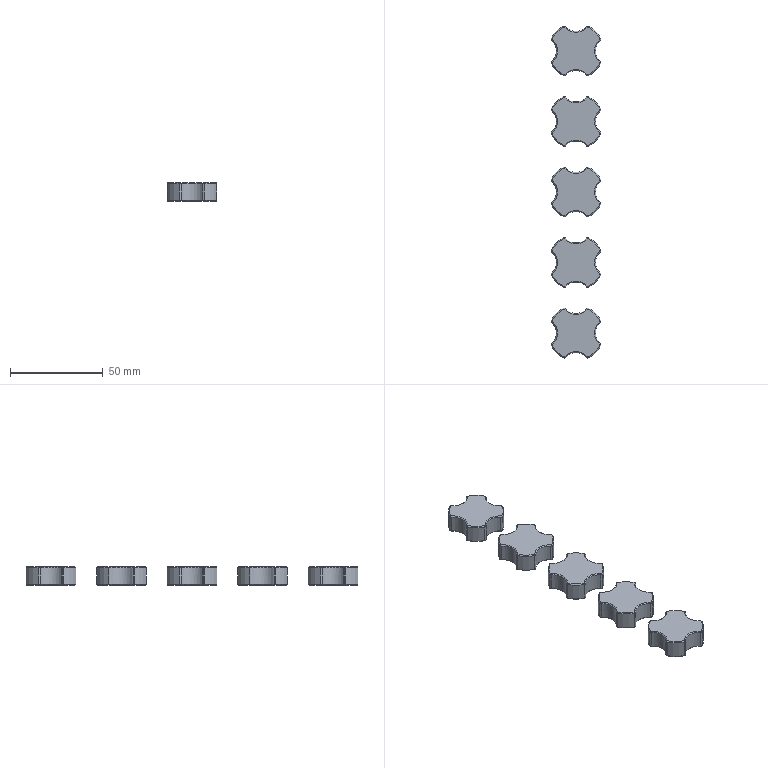NC program | NX | posted with a generic post | part box 26.875 x 178.875 x 10 mm
Lines 9926 to 10509 of 10509:
(ZLEVEL_PROFILE_COPY_1_COPY , TOOL : D10JING)
N19844 T14 M6
N19846 G54
N19848 G17 G0 G90 X8.62 Y19.085 S9500 M3
N19850 G43 Z30. H14
N19852 Z-9.
N19854 G94 G1 Z-10. F1000.
N19856 X8.642 Y18.61
N19858 G3 X9.182 Y17.768 R1.
N19860 G2 X17.768 Y9.182 R20. F1200.
N19862 X16.364 Y1.89 R6.
N19864 G3 X16.364 Y-1.89 R2.5
N19866 G2 X17.768 Y-9.182 R6.
N19868 X9.182 Y-17.768 R20.
N19870 X1.89 Y-16.364 R6.
N19872 G3 X-1.89 Y-16.364 R2.5
N19874 G2 X-9.182 Y-17.768 R6.
N19876 X-17.768 Y-9.182 R20.
N19878 X-16.364 Y-1.89 R6.
N19880 G3 X-16.364 Y1.89 R2.5
N19882 G2 X-17.768 Y9.182 R6.
N19884 X-9.182 Y17.768 R20.
N19886 X-1.89 Y16.364 R6.
N19888 G3 X1.89 Y16.364 R2.5
N19890 G2 X9.182 Y17.768 R6.
N19892 G3 X10.181 Y17.814 R1.
N19894 G1 X10.637 Y18.107
N19896 Z-9.
N19898 G0 Z53.
N19900 X-67.38 Y19.085
N19902 Z-9.
N19904 G1 Z-10. F1000.
N19906 X-67.358 Y18.61
N19908 G3 X-66.818 Y17.768 R1.
N19910 G2 X-58.232 Y9.182 R20. F1200.
N19912 X-59.636 Y1.89 R6.
N19914 G3 X-59.636 Y-1.89 R2.5
N19916 G2 X-58.232 Y-9.182 R6.
N19918 X-66.818 Y-17.768 R20.
N19920 X-74.11 Y-16.364 R6.
N19922 G3 X-77.89 Y-16.364 R2.5
N19924 G2 X-85.182 Y-17.768 R6.
N19926 X-93.768 Y-9.182 R20.
N19928 X-92.364 Y-1.89 R6.
N19930 G3 X-92.364 Y1.89 R2.5
N19932 G2 X-93.768 Y9.182 R6.
N19934 X-85.182 Y17.768 R20.
N19936 X-77.89 Y16.364 R6.
N19938 G3 X-74.11 Y16.364 R2.5
N19940 G2 X-66.818 Y17.768 R6.
N19942 G3 X-65.819 Y17.814 R1.
N19944 G1 X-65.363 Y18.107
N19946 Z-9.
N19948 G0 Z53.
N19950 X19. Y8.863
N19952 Z-9.
N19954 G1 Z-10. F1000.
N19956 X19.39 Y8.642
N19958 G3 X20.232 Y9.182 R1.
N19960 G2 X28.818 Y17.768 R20. F1200.
N19962 X36.11 Y16.364 R6.
N19964 G3 X39.89 Y16.364 R2.5
N19966 G2 X47.182 Y17.768 R6.
N19968 X55.768 Y9.182 R20.
N19970 X54.364 Y1.89 R6.
N19972 G3 X54.364 Y-1.89 R2.5
N19974 G2 X55.768 Y-9.182 R6.
N19976 X47.182 Y-17.768 R20.
N19978 X39.89 Y-16.364 R6.
N19980 G3 X36.11 Y-16.364 R2.5
N19982 G2 X28.818 Y-17.768 R6.
N19984 X20.232 Y-9.182 R20.
N19986 X21.636 Y-1.89 R6.
N19988 G3 X21.636 Y1.89 R2.5
N19990 G2 X20.232 Y9.182 R6.
N19992 G3 X20.186 Y10.181 R1.
N19994 G1 X19.893 Y10.637
N19996 Z-9.
N19998 G0 Z53.
N20000 X57. Y8.863
N20002 Z-9.
N20004 G1 Z-10. F1000.
N20006 X57.39 Y8.642
N20008 G3 X58.232 Y9.182 R1.
N20010 G2 X66.818 Y17.768 R20. F1200.
N20012 X74.11 Y16.364 R6.
N20014 G3 X77.89 Y16.364 R2.5
N20016 G2 X85.182 Y17.768 R6.
N20018 X93.768 Y9.182 R20.
N20020 X92.364 Y1.89 R6.
N20022 G3 X92.364 Y-1.89 R2.5
N20024 G2 X93.768 Y-9.182 R6.
N20026 X85.182 Y-17.768 R20.
N20028 X77.89 Y-16.364 R6.
N20030 G3 X74.11 Y-16.364 R2.5
N20032 G2 X66.818 Y-17.768 R6.
N20034 X58.232 Y-9.182 R20.
N20036 X59.636 Y-1.89 R6.
N20038 G3 X59.636 Y1.89 R2.5
N20040 G2 X58.232 Y9.182 R6.
N20042 G3 X58.186 Y10.181 R1.
N20044 G1 X57.893 Y10.637
N20046 Z-9.
N20048 G0 Z53.
N20050 X-19. Y-8.863
N20052 Z-9.
N20054 G1 Z-10. F1000.
N20056 X-19.39 Y-8.642
N20058 G3 X-20.232 Y-9.182 R1.
N20060 G2 X-28.818 Y-17.768 R20. F1200.
N20062 X-36.11 Y-16.364 R6.
N20064 G3 X-39.89 Y-16.364 R2.5
N20066 G2 X-47.182 Y-17.768 R6.
N20068 X-55.768 Y-9.182 R20.
N20070 X-54.364 Y-1.89 R6.
N20072 G3 X-54.364 Y1.89 R2.5
N20074 G2 X-55.768 Y9.182 R6.
N20076 X-47.182 Y17.768 R20.
N20078 X-39.89 Y16.364 R6.
N20080 G3 X-36.11 Y16.364 R2.5
N20082 G2 X-28.818 Y17.768 R6.
N20084 X-20.232 Y9.182 R20.
N20086 X-21.636 Y1.89 R6.
N20088 G3 X-21.636 Y-1.89 R2.5
N20090 G2 X-20.232 Y-9.182 R6.
N20092 G3 X-20.186 Y-10.181 R1.
N20094 G1 X-19.893 Y-10.637
N20096 Z-9.
N20098 G0 Z30.
N20100 M5
(HOLE_MILLING , TOOL : D3)
N20102 T17 M6
N20104 G54
N20106 G17 G0 G90 X-76. Y0. S9500 M3
N20108 G43 Z30. H17
N20110 Z0.5
N20112 G94 G3 X-75.8 Y0.2 R0.2 F1150.
N20114 X-76. Y0.4 R0.2
N20116 X-76. Y0.4 Z0.25 I0. J-0.4
N20118 X-76. Y0.4 Z0. I0. J-0.4
N20120 X-76. Y0.4 Z-0.25 I0. J-0.4
N20122 X-76. Y0.4 Z-0.5 I0. J-0.4
N20124 X-76. Y0.4 Z-0.75 I0. J-0.4
N20126 X-76. Y0.4 Z-1. I0. J-0.4
N20128 X-76. Y0.4 Z-1.25 I0. J-0.4
N20130 X-76. Y0.4 Z-1.5 I0. J-0.4
N20132 X-76. Y0.4 Z-1.75 I0. J-0.4
N20134 X-76. Y0.4 Z-2. I0. J-0.4
N20136 X-76. Y0.4 Z-2.25 I0. J-0.4
N20138 X-76. Y0.4 Z-2.5 I0. J-0.4
N20140 X-76. Y0.4 Z-2.75 I0. J-0.4
N20142 X-76. Y0.4 Z-3. I0. J-0.4
N20144 X-76. Y0.4 Z-3.25 I0. J-0.4
N20146 X-76. Y0.4 Z-3.5 I0. J-0.4
N20148 X-76. Y0.4 Z-3.75 I0. J-0.4
N20150 X-76. Y0.4 Z-4. I0. J-0.4
N20152 X-76. Y0.4 Z-4.25 I0. J-0.4
N20154 X-76. Y0.4 Z-4.5 I0. J-0.4
N20156 X-76. Y0.4 Z-4.75 I0. J-0.4
N20158 X-76. Y0.4 Z-5. I0. J-0.4
N20160 X-76. Y0.4 Z-5.25 I0. J-0.4
N20162 X-76. Y0.4 Z-5.5 I0. J-0.4
N20164 X-76. Y0.4 Z-5.75 I0. J-0.4
N20166 X-76. Y0.4 Z-6. I0. J-0.4
N20168 X-76. Y0.4 Z-6.25 I0. J-0.4
N20170 X-76. Y0.4 Z-6.5 I0. J-0.4
N20172 X-76. Y0.4 Z-6.75 I0. J-0.4
N20174 X-76. Y0.4 Z-7. I0. J-0.4
N20176 X-76.4 Y0. R0.4
N20178 X-76. Y0.4 R-0.4
N20180 X-76.2 Y0.2 R0.2
N20182 X-76. Y0. R0.2
N20184 G0 Z30.
N20186 X-38.
N20188 Z0.5
N20190 G3 X-37.8 Y0.2 R0.2
N20192 X-38. Y0.4 R0.2
N20194 X-38. Y0.4 Z0.25 I0. J-0.4
N20196 X-38. Y0.4 Z0. I0. J-0.4
N20198 X-38. Y0.4 Z-0.25 I0. J-0.4
N20200 X-38. Y0.4 Z-0.5 I0. J-0.4
N20202 X-38. Y0.4 Z-0.75 I0. J-0.4
N20204 X-38. Y0.4 Z-1. I0. J-0.4
N20206 X-38. Y0.4 Z-1.25 I0. J-0.4
N20208 X-38. Y0.4 Z-1.5 I0. J-0.4
N20210 X-38. Y0.4 Z-1.75 I0. J-0.4
N20212 X-38. Y0.4 Z-2. I0. J-0.4
N20214 X-38. Y0.4 Z-2.25 I0. J-0.4
N20216 X-38. Y0.4 Z-2.5 I0. J-0.4
N20218 X-38. Y0.4 Z-2.75 I0. J-0.4
N20220 X-38. Y0.4 Z-3. I0. J-0.4
N20222 X-38. Y0.4 Z-3.25 I0. J-0.4
N20224 X-38. Y0.4 Z-3.5 I0. J-0.4
N20226 X-38. Y0.4 Z-3.75 I0. J-0.4
N20228 X-38. Y0.4 Z-4. I0. J-0.4
N20230 X-38. Y0.4 Z-4.25 I0. J-0.4
N20232 X-38. Y0.4 Z-4.5 I0. J-0.4
N20234 X-38. Y0.4 Z-4.75 I0. J-0.4
N20236 X-38. Y0.4 Z-5. I0. J-0.4
N20238 X-38. Y0.4 Z-5.25 I0. J-0.4
N20240 X-38. Y0.4 Z-5.5 I0. J-0.4
N20242 X-38. Y0.4 Z-5.75 I0. J-0.4
N20244 X-38. Y0.4 Z-6. I0. J-0.4
N20246 X-38. Y0.4 Z-6.25 I0. J-0.4
N20248 X-38. Y0.4 Z-6.5 I0. J-0.4
N20250 X-38. Y0.4 Z-6.75 I0. J-0.4
N20252 X-38. Y0.4 Z-7. I0. J-0.4
N20254 X-38.4 Y0. R0.4
N20256 X-38. Y0.4 R-0.4
N20258 X-38.2 Y0.2 R0.2
N20260 X-38. Y0. R0.2
N20262 G0 Z30.
N20264 X0.
N20266 Z0.5
N20268 G3 X0.2 Y0.2 R0.2
N20270 X0. Y0.4 R0.2
N20272 X0. Y0.4 Z0.25 I0. J-0.4
N20274 X0. Y0.4 Z0. I0. J-0.4
N20276 X0. Y0.4 Z-0.25 I0. J-0.4
N20278 X0. Y0.4 Z-0.5 I0. J-0.4
N20280 X0. Y0.4 Z-0.75 I0. J-0.4
N20282 X0. Y0.4 Z-1. I0. J-0.4
N20284 X0. Y0.4 Z-1.25 I0. J-0.4
N20286 X0. Y0.4 Z-1.5 I0. J-0.4
N20288 X0. Y0.4 Z-1.75 I0. J-0.4
N20290 X0. Y0.4 Z-2. I0. J-0.4
N20292 X0. Y0.4 Z-2.25 I0. J-0.4
N20294 X0. Y0.4 Z-2.5 I0. J-0.4
N20296 X0. Y0.4 Z-2.75 I0. J-0.4
N20298 X0. Y0.4 Z-3. I0. J-0.4
N20300 X0. Y0.4 Z-3.25 I0. J-0.4
N20302 X0. Y0.4 Z-3.5 I0. J-0.4
N20304 X0. Y0.4 Z-3.75 I0. J-0.4
N20306 X0. Y0.4 Z-4. I0. J-0.4
N20308 X0. Y0.4 Z-4.25 I0. J-0.4
N20310 X0. Y0.4 Z-4.5 I0. J-0.4
N20312 X0. Y0.4 Z-4.75 I0. J-0.4
N20314 X0. Y0.4 Z-5. I0. J-0.4
N20316 X0. Y0.4 Z-5.25 I0. J-0.4
N20318 X0. Y0.4 Z-5.5 I0. J-0.4
N20320 X0. Y0.4 Z-5.75 I0. J-0.4
N20322 X0. Y0.4 Z-6. I0. J-0.4
N20324 X0. Y0.4 Z-6.25 I0. J-0.4
N20326 X0. Y0.4 Z-6.5 I0. J-0.4
N20328 X0. Y0.4 Z-6.75 I0. J-0.4
N20330 X0. Y0.4 Z-7. I0. J-0.4
N20332 X-0.4 Y0. R0.4
N20334 X0. Y0.4 R-0.4
N20336 X-0.2 Y0.2 R0.2
N20338 X0. Y0. R0.2
N20340 G0 Z30.
N20342 X38.
N20344 Z0.5
N20346 G3 X38.2 Y0.2 R0.2
N20348 X38. Y0.4 R0.2
N20350 X38. Y0.4 Z0.25 I0. J-0.4
N20352 X38. Y0.4 Z0. I0. J-0.4
N20354 X38. Y0.4 Z-0.25 I0. J-0.4
N20356 X38. Y0.4 Z-0.5 I0. J-0.4
N20358 X38. Y0.4 Z-0.75 I0. J-0.4
N20360 X38. Y0.4 Z-1. I0. J-0.4
N20362 X38. Y0.4 Z-1.25 I0. J-0.4
N20364 X38. Y0.4 Z-1.5 I0. J-0.4
N20366 X38. Y0.4 Z-1.75 I0. J-0.4
N20368 X38. Y0.4 Z-2. I0. J-0.4
N20370 X38. Y0.4 Z-2.25 I0. J-0.4
N20372 X38. Y0.4 Z-2.5 I0. J-0.4
N20374 X38. Y0.4 Z-2.75 I0. J-0.4
N20376 X38. Y0.4 Z-3. I0. J-0.4
N20378 X38. Y0.4 Z-3.25 I0. J-0.4
N20380 X38. Y0.4 Z-3.5 I0. J-0.4
N20382 X38. Y0.4 Z-3.75 I0. J-0.4
N20384 X38. Y0.4 Z-4. I0. J-0.4
N20386 X38. Y0.4 Z-4.25 I0. J-0.4
N20388 X38. Y0.4 Z-4.5 I0. J-0.4
N20390 X38. Y0.4 Z-4.75 I0. J-0.4
N20392 X38. Y0.4 Z-5. I0. J-0.4
N20394 X38. Y0.4 Z-5.25 I0. J-0.4
N20396 X38. Y0.4 Z-5.5 I0. J-0.4
N20398 X38. Y0.4 Z-5.75 I0. J-0.4
N20400 X38. Y0.4 Z-6. I0. J-0.4
N20402 X38. Y0.4 Z-6.25 I0. J-0.4
N20404 X38. Y0.4 Z-6.5 I0. J-0.4
N20406 X38. Y0.4 Z-6.75 I0. J-0.4
N20408 X38. Y0.4 Z-7. I0. J-0.4
N20410 X37.6 Y0. R0.4
N20412 X38. Y0.4 R-0.4
N20414 X37.8 Y0.2 R0.2
N20416 X38. Y0. R0.2
N20418 G0 Z30.
N20420 X76.
N20422 Z0.5
N20424 G3 X76.2 Y0.2 R0.2
N20426 X76. Y0.4 R0.2
N20428 X76. Y0.4 Z0.25 I0. J-0.4
N20430 X76. Y0.4 Z0. I0. J-0.4
N20432 X76. Y0.4 Z-0.25 I0. J-0.4
N20434 X76. Y0.4 Z-0.5 I0. J-0.4
N20436 X76. Y0.4 Z-0.75 I0. J-0.4
N20438 X76. Y0.4 Z-1. I0. J-0.4
N20440 X76. Y0.4 Z-1.25 I0. J-0.4
N20442 X76. Y0.4 Z-1.5 I0. J-0.4
N20444 X76. Y0.4 Z-1.75 I0. J-0.4
N20446 X76. Y0.4 Z-2. I0. J-0.4
N20448 X76. Y0.4 Z-2.25 I0. J-0.4
N20450 X76. Y0.4 Z-2.5 I0. J-0.4
N20452 X76. Y0.4 Z-2.75 I0. J-0.4
N20454 X76. Y0.4 Z-3. I0. J-0.4
N20456 X76. Y0.4 Z-3.25 I0. J-0.4
N20458 X76. Y0.4 Z-3.5 I0. J-0.4
N20460 X76. Y0.4 Z-3.75 I0. J-0.4
N20462 X76. Y0.4 Z-4. I0. J-0.4
N20464 X76. Y0.4 Z-4.25 I0. J-0.4
N20466 X76. Y0.4 Z-4.5 I0. J-0.4
N20468 X76. Y0.4 Z-4.75 I0. J-0.4
N20470 X76. Y0.4 Z-5. I0. J-0.4
N20472 X76. Y0.4 Z-5.25 I0. J-0.4
N20474 X76. Y0.4 Z-5.5 I0. J-0.4
N20476 X76. Y0.4 Z-5.75 I0. J-0.4
N20478 X76. Y0.4 Z-6. I0. J-0.4
N20480 X76. Y0.4 Z-6.25 I0. J-0.4
N20482 X76. Y0.4 Z-6.5 I0. J-0.4
N20484 X76. Y0.4 Z-6.75 I0. J-0.4
N20486 X76. Y0.4 Z-7. I0. J-0.4
N20488 X75.6 Y0. R0.4
N20490 X76. Y0.4 R-0.4
N20492 X75.8 Y0.2 R0.2
N20494 X76. Y0. R0.2
N20496 G0 Z30.
N20498 M5
(PLANAR_MILL_COPY_COPY_COPY_COPY , TOOL : D6A45)
N20500 T01 M6
N20502 G54
N20504 G17 G0 G90 X-76.5 Y0.866 S9500 M3
N20506 G43 Z30. H1
N20508 Z0.
N20510 G94 G1 Z-1.5 F1250.
N20512 G3 X-77. Y0. R1.
N20514 X-76. Y-1. R1.
N20516 X-77. Y0. R-1.
N20518 X-76.5 Y-0.866 R1.
N20520 G1 Z0.
N20522 G0 Z30.
N20524 X-88.
N20526 Z0.
N20528 G1 Z-1.5
N20530 G3 X-87.5 Y0. R1.
N20532 X-89.746 Y4.915 R6.5
N20534 G2 X-90.214 Y7.345 R2.
N20536 X-83.345 Y14.214 R16.
N20538 X-80.915 Y13.746 R2.
N20540 G3 X-71.085 Y13.746 R6.5
N20542 G2 X-68.655 Y14.214 R2.
N20544 X-61.786 Y7.345 R16.
N20546 X-62.254 Y4.915 R2.
N20548 G3 X-62.254 Y-4.915 R6.5
N20550 G2 X-61.786 Y-7.345 R2.
N20552 X-68.655 Y-14.214 R16.
N20554 X-71.085 Y-13.746 R2.
N20556 G3 X-80.915 Y-13.746 R6.5
N20558 G2 X-83.345 Y-14.214 R2.
N20560 X-90.214 Y-7.345 R16.
N20562 X-89.746 Y-4.915 R2.
N20564 G3 X-87.5 Y0. R6.5
N20566 X-88. Y0.866 R1.
N20568 G1 Z0.
N20570 G0 Z30.
N20572 X-37.134 Y0.5
N20574 Z0.
N20576 G1 Z-1.5
N20578 G3 X-38. Y1. R1.
N20580 X-39. Y0. R1.
N20582 X-38. Y1. R-1.
N20584 X-38.866 Y0.5 R1.
N20586 G1 Z0.
N20588 G0 Z30.
N20590 X-37.134 Y-12.
N20592 Z0.
N20594 G1 Z-1.5
N20596 G3 X-38. Y-11.5 R1.
N20598 X-42.915 Y-13.746 R6.5
N20600 G2 X-45.345 Y-14.214 R2.
N20602 X-52.214 Y-7.345 R16.
N20604 X-51.746 Y-4.915 R2.
N20606 G3 X-51.746 Y4.915 R6.5
N20608 G2 X-52.214 Y7.345 R2.
N20610 X-45.345 Y14.214 R16.
N20612 X-42.915 Y13.746 R2.
N20614 G3 X-33.085 Y13.746 R6.5
N20616 G2 X-30.655 Y14.214 R2.
N20618 X-23.786 Y7.345 R16.
N20620 X-24.254 Y4.915 R2.
N20622 G3 X-24.254 Y-4.915 R6.5
N20624 G2 X-23.786 Y-7.345 R2.
N20626 X-30.655 Y-14.214 R16.
N20628 X-33.085 Y-13.746 R2.
N20630 G3 X-38. Y-11.5 R6.5
N20632 X-38.866 Y-12. R1.
N20634 G1 Z0.
N20636 G0 Z30.
N20638 X0.866 Y0.5
N20640 Z0.
N20642 G1 Z-1.5
N20644 G3 X0. Y1. R1.
N20646 X-1. Y0. R1.
N20648 X0. Y1. R-1.
N20650 X-0.866 Y0.5 R1.
N20652 G1 Z0.
N20654 G0 Z30.
N20656 X0.866 Y-12.
N20658 Z0.
N20660 G1 Z-1.5
N20662 G3 X0. Y-11.5 R1.
N20664 X-4.915 Y-13.746 R6.5
N20666 G2 X-7.345 Y-14.214 R2.
N20668 X-14.214 Y-7.345 R16.
N20670 X-13.746 Y-4.915 R2.
N20672 G3 X-13.746 Y4.915 R6.5
N20674 G2 X-14.214 Y7.345 R2.
N20676 X-7.345 Y14.214 R16.
N20678 X-4.915 Y13.746 R2.
N20680 G3 X4.915 Y13.746 R6.5
N20682 G2 X7.345 Y14.214 R2.
N20684 X14.214 Y7.345 R16.
N20686 X13.746 Y4.915 R2.
N20688 G3 X13.746 Y-4.915 R6.5
N20690 G2 X14.214 Y-7.345 R2.
N20692 X7.345 Y-14.214 R16.
N20694 X4.915 Y-13.746 R2.
N20696 G3 X0. Y-11.5 R6.5
N20698 X-0.866 Y-12. R1.
N20700 G1 Z0.
N20702 G0 Z30.
N20704 X38.866 Y0.5
N20706 Z0.
N20708 G1 Z-1.5
N20710 G3 X38. Y1. R1.
N20712 X37. Y0. R1.
N20714 X38. Y1. R-1.
N20716 X37.134 Y0.5 R1.
N20718 G1 Z0.
N20720 G0 Z30.
N20722 X38.866 Y-12.
N20724 Z0.
N20726 G1 Z-1.5
N20728 G3 X38. Y-11.5 R1.
N20730 X33.085 Y-13.746 R6.5
N20732 G2 X30.655 Y-14.214 R2.
N20734 X23.786 Y-7.345 R16.
N20736 X24.254 Y-4.915 R2.
N20738 G3 X24.254 Y4.915 R6.5
N20740 G2 X23.786 Y7.345 R2.
N20742 X30.655 Y14.214 R16.
N20744 X33.085 Y13.746 R2.
N20746 G3 X42.915 Y13.746 R6.5
N20748 G2 X45.345 Y14.214 R2.
N20750 X52.214 Y7.345 R16.
N20752 X51.746 Y4.915 R2.
N20754 G3 X51.746 Y-4.915 R6.5
N20756 G2 X52.214 Y-7.345 R2.
N20758 X45.345 Y-14.214 R16.
N20760 X42.915 Y-13.746 R2.
N20762 G3 X38. Y-11.5 R6.5
N20764 X37.134 Y-12. R1.
N20766 G1 Z0.
N20768 G0 Z30.
N20770 X76.866 Y0.5
N20772 Z0.
N20774 G1 Z-1.5
N20776 G3 X76. Y1. R1.
N20778 X75. Y0. R1.
N20780 X76. Y1. R-1.
N20782 X75.134 Y0.5 R1.
N20784 G1 Z0.
N20786 G0 Z30.
N20788 X76.866 Y-12.
N20790 Z0.
N20792 G1 Z-1.5
N20794 G3 X76. Y-11.5 R1.
N20796 X71.085 Y-13.746 R6.5
N20798 G2 X68.655 Y-14.214 R2.
N20800 X61.786 Y-7.345 R16.
N20802 X62.254 Y-4.915 R2.
N20804 G3 X62.254 Y4.915 R6.5
N20806 G2 X61.786 Y7.345 R2.
N20808 X68.655 Y14.214 R16.
N20810 X71.085 Y13.746 R2.
N20812 G3 X80.915 Y13.746 R6.5
N20814 G2 X83.345 Y14.214 R2.
N20816 X90.214 Y7.345 R16.
N20818 X89.746 Y4.915 R2.
N20820 G3 X89.746 Y-4.915 R6.5
N20822 G2 X90.214 Y-7.345 R2.
N20824 X83.345 Y-14.214 R16.
N20826 X80.915 Y-13.746 R2.
N20828 G3 X76. Y-11.5 R6.5
N20830 X75.134 Y-12. R1.
N20832 G1 Z0.
N20834 G0 Z30.
N20836 M5
(刀补17 , TOOL : D3)
N20838 T17 M6
N20840 G54
N20842 G17 G0 G90 X-76. Y0. S9500 M3
N20844 G43 Z30. H17
N20846 Z0.5
N20848 G41 G94 G1 X-75.904 Y0.027 F1150. D17
N20850 G3 X-76. Y0.45 R0.222
N20852 X-76. Y0.45 Z-1.5 I0. J-0.45
N20854 X-76. Y0.45 Z-3.5 I0. J-0.45
N20856 X-76. Y0.45 Z-5.5 I0. J-0.45
N20858 X-75.55 Y0. Z-7. R-0.45
N20860 X-76. Y0.45 R0.45
N20862 X-75.55 Y0. R-0.45
N20864 X-75.973 Y0.096 R0.222
N20866 G40
N20868 G1 X-76. Y0.
N20870 G0 Z30.
N20872 X-38.
N20874 Z0.5
N20876 G41 G1 X-37.904 Y0.027
N20878 G3 X-38. Y0.45 R0.222
N20880 X-38. Y0.45 Z-1.5 I0. J-0.45
N20882 X-38. Y0.45 Z-3.5 I0. J-0.45
N20884 X-38. Y0.45 Z-5.5 I0. J-0.45
N20886 X-37.55 Y0. Z-7. R-0.45
N20888 X-38. Y0.45 R0.45
N20890 X-37.55 Y0. R-0.45
N20892 X-37.973 Y0.096 R0.222
N20894 G40
N20896 G1 X-38. Y0.
N20898 G0 Z30.
N20900 X0.
N20902 Z0.5
N20904 G41 G1 X0.096 Y0.027
N20906 G3 X0. Y0.45 R0.222
N20908 X0. Y0.45 Z-1.5 I0. J-0.45
N20910 X0. Y0.45 Z-3.5 I0. J-0.45
N20912 X0. Y0.45 Z-5.5 I0. J-0.45
N20914 X0.45 Y0. Z-7. R-0.45
N20916 X0. Y0.45 R0.45
N20918 X0.45 Y0. R-0.45
N20920 X0.027 Y0.096 R0.222
N20922 G40
N20924 G1 X0. Y0.
N20926 G0 Z30.
N20928 X38.
N20930 Z0.5
N20932 G41 G1 X38.096 Y0.027
N20934 G3 X38. Y0.45 R0.222
N20936 X38. Y0.45 Z-1.5 I0. J-0.45
N20938 X38. Y0.45 Z-3.5 I0. J-0.45
N20940 X38. Y0.45 Z-5.5 I0. J-0.45
N20942 X38.45 Y0. Z-7. R-0.45
N20944 X38. Y0.45 R0.45
N20946 X38.45 Y0. R-0.45
N20948 X38.027 Y0.096 R0.222
N20950 G40
N20952 G1 X38. Y0.
N20954 G0 Z30.
N20956 X76.
N20958 Z0.5
N20960 G41 G1 X76.096 Y0.027
N20962 G3 X76. Y0.45 R0.222
N20964 X76. Y0.45 Z-1.5 I0. J-0.45
N20966 X76. Y0.45 Z-3.5 I0. J-0.45
N20968 X76. Y0.45 Z-5.5 I0. J-0.45
N20970 X76.45 Y0. Z-7. R-0.45
N20972 X76. Y0.45 R0.45
N20974 X76.45 Y0. R-0.45
N20976 X76.027 Y0.096 R0.222
N20978 G40
N20980 G1 X76. Y0.
N20982 G0 Z30.
N20984 M5
N20986 M2